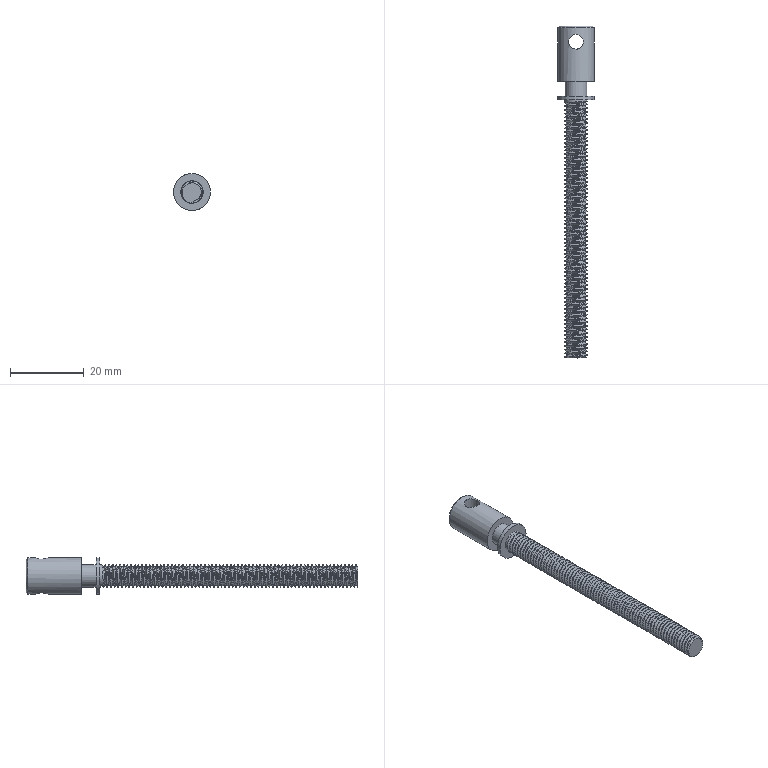Part | NX | features EXTRUDE 5, SKETCH 4, LINE 2, UNITE 2, CHAMFER 1, DATUM_CSYS 1, INTERSECTION_CURVES 1, THREADS 1 | 1 solid | 16 faces | box 10 x 90 x 10 mm | volume 2885 mm3 | cylinder 6 | plane 6 | spline 3 | cone 1 | commonest cylinder face diameters 6 x2 10 x2 4 x1 5 x1